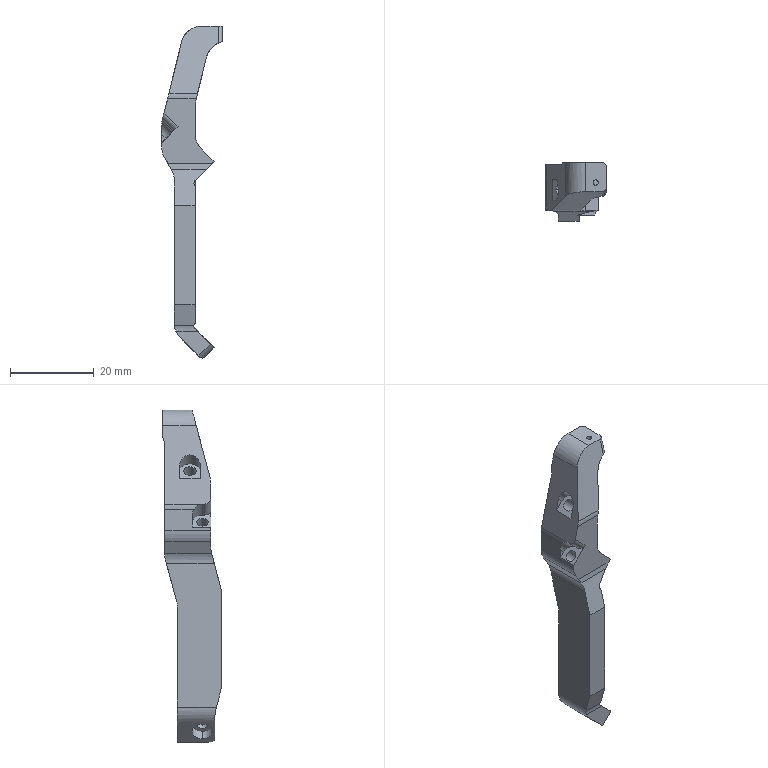NC program | NX | posted by the shop | part box 14.5 x 14 x 79.438 mm
Lines 12095 to 13169 of 13169:
T04 M6 ( D4-12-D4-50-3T-rough )
M41
M51
G90 G54 G00 B90. C225.
M40
M50
G54 G00 X-166.572 Y-9.003 S3000 M03
G43 H04 Z-115.926 M08
Z-148.07
G01 Z-150.07 F400.
Y-13.003
Y-15.568
G03 X-166.122 Y-16.018 R0.45
X-165.672 Y-15.568 R0.45
G01 Y-13.003
Y-9.003
Z-148.07
G00 X-166.572 Z-148.17
G01 Z-150.17
Y-13.003
Y-15.568
G03 X-166.122 Y-16.018 R0.45
X-165.672 Y-15.568 R0.45
G01 Y-13.003
Y-9.003
Z-148.17
G00 X-166.572 Z-148.27
G01 Z-150.27
Y-13.003
Y-15.568
G03 X-166.122 Y-16.018 R0.45
X-165.672 Y-15.568 R0.45
G01 Y-13.003
Y-9.003
Z-148.27
G00 X-166.572 Z-148.37
G01 Z-150.37
Y-13.003
Y-15.568
G03 X-166.122 Y-16.018 R0.45
X-165.672 Y-15.568 R0.45
G01 Y-13.003
Y-9.003
Z-148.37
G00 X-166.572 Z-148.47
G01 Z-150.47
Y-13.003
Y-15.568
G03 X-166.122 Y-16.018 R0.45
X-165.672 Y-15.568 R0.45
G01 Y-13.003
Y-9.003
Z-148.47
G00 X-166.572 Z-148.57
G01 Z-150.57
Y-13.003
Y-15.568
G03 X-166.122 Y-16.018 R0.45
X-165.672 Y-15.568 R0.45
G01 Y-13.003
Y-9.003
Z-148.57
G00 X-166.572 Z-148.67
G01 Z-150.67
Y-13.003
Y-15.568
G03 X-166.122 Y-16.018 R0.45
X-165.672 Y-15.568 R0.45
G01 Y-13.003
Y-9.003
Z-148.67
G00 X-166.572 Z-148.77
G01 Z-150.77
Y-13.003
Y-15.568
G03 X-166.122 Y-16.018 R0.45
X-165.672 Y-15.568 R0.45
G01 Y-13.003
Y-9.003
Z-148.77
G00 X-166.572 Z-148.87
G01 Z-150.87
Y-13.003
Y-15.568
G03 X-166.122 Y-16.018 R0.45
X-165.672 Y-15.568 R0.45
G01 Y-13.003
Y-9.003
Z-148.87
G00 X-166.572 Z-148.97
G01 Z-150.97
Y-13.003
Y-15.568
G03 X-166.122 Y-16.018 R0.45
X-165.672 Y-15.568 R0.45
G01 Y-13.003
Y-9.003
Z-148.97
G00 X-166.572 Z-149.07
G01 Z-151.07
Y-13.003
Y-15.568
G03 X-166.122 Y-16.018 R0.45
X-165.672 Y-15.568 R0.45
G01 Y-13.003
Y-9.003
Z-149.07
G00 X-166.572 Z-149.17
G01 Z-151.17
Y-13.003
Y-15.568
G03 X-166.122 Y-16.018 R0.45
X-165.672 Y-15.568 R0.45
G01 Y-13.003
Y-9.003
Z-149.17
G00 X-166.572 Z-149.27
G01 Z-151.27
Y-13.003
Y-15.568
G03 X-166.122 Y-16.018 R0.45
X-165.672 Y-15.568 R0.45
G01 Y-13.003
Y-9.003
Z-149.27
G00 X-166.572 Z-149.37
G01 Z-151.37
Y-13.003
Y-15.568
G03 X-166.122 Y-16.018 R0.45
X-165.672 Y-15.568 R0.45
G01 Y-13.003
Y-9.003
Z-149.37
G00 X-166.572 Z-149.47
G01 Z-151.47
Y-13.003
Y-15.568
G03 X-166.122 Y-16.018 R0.45
X-165.672 Y-15.568 R0.45
G01 Y-13.003
Y-9.003
Z-149.47
G00 X-166.572 Z-149.57
G01 Z-151.57
Y-13.003
Y-15.568
G03 X-166.122 Y-16.018 R0.45
X-165.672 Y-15.568 R0.45
G01 Y-13.003
Y-9.003
Z-149.57
G00 X-166.572 Z-149.67
G01 Z-151.67
Y-13.003
Y-15.568
G03 X-166.122 Y-16.018 R0.45
X-165.672 Y-15.568 R0.45
G01 Y-13.003
Y-9.003
Z-149.67
G00 X-166.572 Z-149.77
G01 Z-151.77
Y-13.003
Y-15.568
G03 X-166.122 Y-16.018 R0.45
X-165.672 Y-15.568 R0.45
G01 Y-13.003
Y-9.003
Z-149.77
G00 X-166.572 Z-149.87
G01 Z-151.87
Y-13.003
Y-15.568
G03 X-166.122 Y-16.018 R0.45
X-165.672 Y-15.568 R0.45
G01 Y-13.003
Y-9.003
Z-149.87
G00 X-166.572 Z-149.97
G01 Z-151.97
Y-13.003
Y-15.568
G03 X-166.122 Y-16.018 R0.45
X-165.672 Y-15.568 R0.45
G01 Y-13.003
Y-9.003
Z-149.97
G00 X-166.572 Z-150.07
G01 Z-152.07
Y-13.003
Y-15.568
G03 X-166.122 Y-16.018 R0.45
X-165.672 Y-15.568 R0.45
G01 Y-13.003
Y-9.003
Z-150.07
G00 X-166.572 Z-150.17
G01 Z-152.17
Y-13.003
Y-15.568
G03 X-166.122 Y-16.018 R0.45
X-165.672 Y-15.568 R0.45
G01 Y-13.003
Y-9.003
Z-150.17
G00 X-166.572 Z-150.27
G01 Z-152.27
Y-13.003
Y-15.568
G03 X-166.122 Y-16.018 R0.45
X-165.672 Y-15.568 R0.45
G01 Y-13.003
Y-9.003
Z-150.27
G00 X-166.572 Z-150.37
G01 Z-152.37
Y-13.003
Y-15.568
G03 X-166.122 Y-16.018 R0.45
X-165.672 Y-15.568 R0.45
G01 Y-13.003
Y-9.003
Z-150.37
G00 X-166.572 Z-150.47
G01 Z-152.47
Y-13.003
Y-15.568
G03 X-166.122 Y-16.018 R0.45
X-165.672 Y-15.568 R0.45
G01 Y-13.003
Y-9.003
Z-150.47
G00 X-166.572 Z-150.57
G01 Z-152.57
Y-13.003
Y-15.568
G03 X-166.122 Y-16.018 R0.45
X-165.672 Y-15.568 R0.45
G01 Y-13.003
Y-9.003
Z-150.57
G00 X-166.572 Z-150.67
G01 Z-152.67
Y-13.003
Y-15.568
G03 X-166.122 Y-16.018 R0.45
X-165.672 Y-15.568 R0.45
G01 Y-13.003
Y-9.003
Z-150.67
G00 X-166.572 Z-150.77
G01 Z-152.77
Y-13.003
Y-15.568
G03 X-166.122 Y-16.018 R0.45
X-165.672 Y-15.568 R0.45
G01 Y-13.003
Y-9.003
Z-150.77
G00 X-166.572 Z-150.87
G01 Z-152.87
Y-13.003
Y-15.568
G03 X-166.122 Y-16.018 R0.45
X-165.672 Y-15.568 R0.45
G01 Y-13.003
Y-9.003
Z-150.87
G00 X-166.572 Z-150.97
G01 Z-152.97
Y-13.003
Y-15.568
G03 X-166.122 Y-16.018 R0.45
X-165.672 Y-15.568 R0.45
G01 Y-13.003
Y-9.003
Z-150.97
G00 X-166.572 Z-151.07
G01 Z-153.07
Y-13.003
Y-15.568
G03 X-166.122 Y-16.018 R0.45
X-165.672 Y-15.568 R0.45
G01 Y-13.003
Y-9.003
Z-151.07
G00 X-166.572 Z-151.17
G01 Z-153.17
Y-13.003
Y-15.568
G03 X-166.122 Y-16.018 R0.45
X-165.672 Y-15.568 R0.45
G01 Y-13.003
Y-9.003
Z-151.17
G00 X-166.572 Z-151.27
G01 Z-153.27
Y-13.003
Y-15.568
G03 X-166.122 Y-16.018 R0.45
X-165.672 Y-15.568 R0.45
G01 Y-13.003
Y-9.003
Z-151.27
G00 X-166.572 Z-151.37
G01 Z-153.37
Y-13.003
Y-15.568
G03 X-166.122 Y-16.018 R0.45
X-165.672 Y-15.568 R0.45
G01 Y-13.003
Y-9.003
Z-151.37
G00 X-166.572 Z-151.42
G01 Z-153.42
Y-13.003
Y-15.568
G03 X-166.122 Y-16.018 R0.45
X-165.672 Y-15.568 R0.45
G01 Y-13.003
Y-9.003
Z-151.42
G00 Z-115.926
G00 X-175.172 Y-11.221
Z-153.57
G01 Z-155.57 F400.
G03 X-173.172 Y-9.221 R2.
G02 X-169.622 Y-5.671 R3.55
G01 X-169.122
G03 X-168.672 Y-5.221 R0.45
G01 Y-5.211
Y-2.711
G03 X-170.672 Y-0.711 R2.
G01 Z-153.57
G00 X-175.172 Y-11.221 Z-153.67
G01 Z-155.67
G03 X-173.172 Y-9.221 R2.
G02 X-169.622 Y-5.671 R3.55
G01 X-169.122
G03 X-168.672 Y-5.221 R0.45
G01 Y-5.211
Y-2.711
G03 X-170.672 Y-0.711 R2.
G01 Z-153.67
G00 X-175.172 Y-11.221 Z-153.77
G01 Z-155.77
G03 X-173.172 Y-9.221 R2.
G02 X-169.622 Y-5.671 R3.55
G01 X-169.122
G03 X-168.672 Y-5.221 R0.45
G01 Y-5.211
Y-2.711
G03 X-170.672 Y-0.711 R2.
G01 Z-153.77
G00 X-175.172 Y-11.221 Z-153.87
G01 Z-155.87
G03 X-173.172 Y-9.221 R2.
G02 X-169.622 Y-5.671 R3.55
G01 X-169.122
G03 X-168.672 Y-5.221 R0.45
G01 Y-5.211
Y-2.711
G03 X-170.672 Y-0.711 R2.
G01 Z-153.87
G00 X-175.172 Y-11.221 Z-153.97
G01 Z-155.97
G03 X-173.172 Y-9.221 R2.
G02 X-169.622 Y-5.671 R3.55
G01 X-169.122
G03 X-168.672 Y-5.221 R0.45
G01 Y-5.211
Y-2.711
G03 X-170.672 Y-0.711 R2.
G01 Z-153.97
G00 X-175.172 Y-11.221 Z-154.07
G01 Z-156.07
G03 X-173.172 Y-9.221 R2.
G02 X-169.622 Y-5.671 R3.55
G01 X-169.122
G03 X-168.672 Y-5.221 R0.45
G01 Y-5.211
Y-2.711
G03 X-170.672 Y-0.711 R2.
G01 Z-154.07
G00 X-175.172 Y-11.221 Z-154.17
G01 Z-156.17
G03 X-173.172 Y-9.221 R2.
G02 X-169.622 Y-5.671 R3.55
G01 X-169.122
G03 X-168.672 Y-5.221 R0.45
G01 Y-5.211
Y-2.711
G03 X-170.672 Y-0.711 R2.
G01 Z-154.17
G00 X-175.172 Y-11.221 Z-154.27
G01 Z-156.27
G03 X-173.172 Y-9.221 R2.
G02 X-169.622 Y-5.671 R3.55
G01 X-169.122
G03 X-168.672 Y-5.221 R0.45
G01 Y-5.211
Y-2.711
G03 X-170.672 Y-0.711 R2.
G01 Z-154.27
G00 X-175.172 Y-11.221 Z-154.37
G01 Z-156.37
G03 X-173.172 Y-9.221 R2.
G02 X-169.622 Y-5.671 R3.55
G01 X-169.122
G03 X-168.672 Y-5.221 R0.45
G01 Y-5.211
Y-2.711
G03 X-170.672 Y-0.711 R2.
G01 Z-154.37
G00 X-175.172 Y-11.221 Z-154.47
G01 Z-156.47
G03 X-173.172 Y-9.221 R2.
G02 X-169.622 Y-5.671 R3.55
G01 X-169.122
G03 X-168.672 Y-5.221 R0.45
G01 Y-5.211
Y-2.711
G03 X-170.672 Y-0.711 R2.
G01 Z-154.47
G00 X-175.172 Y-11.221 Z-154.57
G01 Z-156.57
G03 X-173.172 Y-9.221 R2.
G02 X-169.622 Y-5.671 R3.55
G01 X-169.122
G03 X-168.672 Y-5.221 R0.45
G01 Y-5.211
Y-2.711
G03 X-170.672 Y-0.711 R2.
G01 Z-154.57
G00 X-175.172 Y-11.221 Z-154.67
G01 Z-156.67
G03 X-173.172 Y-9.221 R2.
G02 X-169.622 Y-5.671 R3.55
G01 X-169.122
G03 X-168.672 Y-5.221 R0.45
G01 Y-5.211
Y-2.711
G03 X-170.672 Y-0.711 R2.
G01 Z-154.67
G00 X-175.172 Y-11.221 Z-154.77
G01 Z-156.77
G03 X-173.172 Y-9.221 R2.
G02 X-169.622 Y-5.671 R3.55
G01 X-169.122
G03 X-168.672 Y-5.221 R0.45
G01 Y-5.211
Y-2.711
G03 X-170.672 Y-0.711 R2.
G01 Z-154.77
G00 X-175.172 Y-11.221 Z-154.87
G01 Z-156.87
G03 X-173.172 Y-9.221 R2.
G02 X-169.622 Y-5.671 R3.55
G01 X-169.122
G03 X-168.672 Y-5.221 R0.45
G01 Y-5.211
Y-2.711
G03 X-170.672 Y-0.711 R2.
G01 Z-154.87
G00 X-175.172 Y-11.221 Z-154.97
G01 Z-156.97
G03 X-173.172 Y-9.221 R2.
G02 X-169.622 Y-5.671 R3.55
G01 X-169.122
G03 X-168.672 Y-5.221 R0.45
G01 Y-5.211
Y-2.711
G03 X-170.672 Y-0.711 R2.
G01 Z-154.97
G00 X-175.172 Y-11.221 Z-155.07
G01 Z-157.07
G03 X-173.172 Y-9.221 R2.
G02 X-169.622 Y-5.671 R3.55
G01 X-169.122
G03 X-168.672 Y-5.221 R0.45
G01 Y-5.211
Y-2.711
G03 X-170.672 Y-0.711 R2.
G01 Z-155.07
G00 X-175.172 Y-11.221 Z-155.17
G01 Z-157.17
G03 X-173.172 Y-9.221 R2.
G02 X-169.622 Y-5.671 R3.55
G01 X-169.122
G03 X-168.672 Y-5.221 R0.45
G01 Y-5.211
Y-2.711
G03 X-170.672 Y-0.711 R2.
G01 Z-155.17
G00 X-175.172 Y-11.221 Z-155.27
G01 Z-157.27
G03 X-173.172 Y-9.221 R2.
G02 X-169.622 Y-5.671 R3.55
G01 X-169.122
G03 X-168.672 Y-5.221 R0.45
G01 Y-5.211
Y-2.711
G03 X-170.672 Y-0.711 R2.
G01 Z-155.27
G00 X-175.172 Y-11.221 Z-155.37
G01 Z-157.37
G03 X-173.172 Y-9.221 R2.
G02 X-169.622 Y-5.671 R3.55
G01 X-169.122
G03 X-168.672 Y-5.221 R0.45
G01 Y-5.211
Y-2.711
G03 X-170.672 Y-0.711 R2.
G01 Z-155.37
G00 X-175.172 Y-11.221 Z-155.47
G01 Z-157.47
G03 X-173.172 Y-9.221 R2.
G02 X-169.622 Y-5.671 R3.55
G01 X-169.122
G03 X-168.672 Y-5.221 R0.45
G01 Y-5.211
Y-2.711
G03 X-170.672 Y-0.711 R2.
G01 Z-155.47
G00 X-175.172 Y-11.221 Z-155.57
G01 Z-157.57
G03 X-173.172 Y-9.221 R2.
G02 X-169.622 Y-5.671 R3.55
G01 X-169.122
G03 X-168.672 Y-5.221 R0.45
G01 Y-5.211
Y-2.711
G03 X-170.672 Y-0.711 R2.
G01 Z-155.57
G00 X-175.172 Y-11.221 Z-155.67
G01 Z-157.67
G03 X-173.172 Y-9.221 R2.
G02 X-169.622 Y-5.671 R3.55
G01 X-169.122
G03 X-168.672 Y-5.221 R0.45
G01 Y-5.211
Y-2.711
G03 X-170.672 Y-0.711 R2.
G01 Z-155.67
G00 X-175.172 Y-11.221 Z-155.77
G01 Z-157.77
G03 X-173.172 Y-9.221 R2.
G02 X-169.622 Y-5.671 R3.55
G01 X-169.122
G03 X-168.672 Y-5.221 R0.45
G01 Y-5.211
Y-2.711
G03 X-170.672 Y-0.711 R2.
G01 Z-155.77
G00 X-175.172 Y-11.221 Z-155.87
G01 Z-157.87
G03 X-173.172 Y-9.221 R2.
G02 X-169.622 Y-5.671 R3.55
G01 X-169.122
G03 X-168.672 Y-5.221 R0.45
G01 Y-5.211
Y-2.711
G03 X-170.672 Y-0.711 R2.
G01 Z-155.87
G00 X-175.172 Y-11.221 Z-155.97
G01 Z-157.97
G03 X-173.172 Y-9.221 R2.
G02 X-169.622 Y-5.671 R3.55
G01 X-169.122
G03 X-168.672 Y-5.221 R0.45
G01 Y-5.211
Y-2.711
G03 X-170.672 Y-0.711 R2.
G01 Z-155.97
G00 X-175.172 Y-11.221 Z-156.07
G01 Z-158.07
G03 X-173.172 Y-9.221 R2.
G02 X-169.622 Y-5.671 R3.55
G01 X-169.122
G03 X-168.672 Y-5.221 R0.45
G01 Y-5.211
Y-2.711
G03 X-170.672 Y-0.711 R2.
G01 Z-156.07
G00 X-175.172 Y-11.221 Z-156.17
G01 Z-158.17
G03 X-173.172 Y-9.221 R2.
G02 X-169.622 Y-5.671 R3.55
G01 X-169.122
G03 X-168.672 Y-5.221 R0.45
G01 Y-5.211
Y-2.711
G03 X-170.672 Y-0.711 R2.
G01 Z-156.17
G00 X-175.172 Y-11.221 Z-156.27
G01 Z-158.27
G03 X-173.172 Y-9.221 R2.
G02 X-169.622 Y-5.671 R3.55
G01 X-169.122
G03 X-168.672 Y-5.221 R0.45
G01 Y-5.211
Y-2.711
G03 X-170.672 Y-0.711 R2.
G01 Z-156.27
G00 X-175.172 Y-11.221 Z-156.37
G01 Z-158.37
G03 X-173.172 Y-9.221 R2.
G02 X-169.622 Y-5.671 R3.55
G01 X-169.122
G03 X-168.672 Y-5.221 R0.45
G01 Y-5.211
Y-2.711
G03 X-170.672 Y-0.711 R2.
G01 Z-156.37
G00 X-175.172 Y-11.221 Z-156.47
G01 Z-158.47
G03 X-173.172 Y-9.221 R2.
G02 X-169.622 Y-5.671 R3.55
G01 X-169.122
G03 X-168.672 Y-5.221 R0.45
G01 Y-5.211
Y-2.711
G03 X-170.672 Y-0.711 R2.
G01 Z-156.47
G00 X-175.172 Y-11.221 Z-156.57
G01 Z-158.57
G03 X-173.172 Y-9.221 R2.
G02 X-169.622 Y-5.671 R3.55
G01 X-169.122
G03 X-168.672 Y-5.221 R0.45
G01 Y-5.211
Y-2.711
G03 X-170.672 Y-0.711 R2.
G01 Z-156.57
G00 X-175.172 Y-11.221 Z-156.67
G01 Z-158.67
G03 X-173.172 Y-9.221 R2.
G02 X-169.622 Y-5.671 R3.55
G01 X-169.122
G03 X-168.672 Y-5.221 R0.45
G01 Y-5.211
Y-2.711
G03 X-170.672 Y-0.711 R2.
G01 Z-156.67
G00 X-175.172 Y-11.221 Z-156.77
G01 Z-158.77
G03 X-173.172 Y-9.221 R2.
G02 X-169.622 Y-5.671 R3.55
G01 X-169.122
G03 X-168.672 Y-5.221 R0.45
G01 Y-5.211
Y-2.711
G03 X-170.672 Y-0.711 R2.
G01 Z-156.77
G00 X-175.172 Y-11.221 Z-156.87
G01 Z-158.87
G03 X-173.172 Y-9.221 R2.
G02 X-169.622 Y-5.671 R3.55
G01 X-169.122
G03 X-168.672 Y-5.221 R0.45
G01 Y-5.211
Y-2.711
G03 X-170.672 Y-0.711 R2.
G01 Z-156.87
G00 X-175.172 Y-11.221 Z-156.97
G01 Z-158.97
G03 X-173.172 Y-9.221 R2.
G02 X-169.622 Y-5.671 R3.55
G01 X-169.122
G03 X-168.672 Y-5.221 R0.45
G01 Y-5.211
Y-2.711
G03 X-170.672 Y-0.711 R2.
G01 Z-156.97
G00 X-175.172 Y-11.221 Z-157.07
G01 Z-159.07
G03 X-173.172 Y-9.221 R2.
G02 X-169.622 Y-5.671 R3.55
G01 X-169.122
G03 X-168.672 Y-5.221 R0.45
G01 Y-5.211
Y-2.711
G03 X-170.672 Y-0.711 R2.
G01 Z-157.07
G00 X-175.172 Y-11.221 Z-157.17
G01 Z-159.17
G03 X-173.172 Y-9.221 R2.
G02 X-169.622 Y-5.671 R3.55
G01 X-169.122
G03 X-168.672 Y-5.221 R0.45
G01 Y-5.211
Y-2.711
G03 X-170.672 Y-0.711 R2.
G01 Z-157.17
G00 X-175.172 Y-11.221 Z-157.27
G01 Z-159.27
G03 X-173.172 Y-9.221 R2.
G02 X-169.622 Y-5.671 R3.55
G01 X-169.122
G03 X-168.672 Y-5.221 R0.45
G01 Y-5.211
Y-2.711
G03 X-170.672 Y-0.711 R2.
G01 Z-157.27
G00 X-175.172 Y-11.221 Z-157.37
G01 Z-159.37
G03 X-173.172 Y-9.221 R2.
G02 X-169.622 Y-5.671 R3.55
G01 X-169.122
G03 X-168.672 Y-5.221 R0.45
G01 Y-5.211
Y-2.711
G03 X-170.672 Y-0.711 R2.
G01 Z-157.37
G00 X-175.172 Y-11.221 Z-157.47
G01 Z-159.47
G03 X-173.172 Y-9.221 R2.
G02 X-169.622 Y-5.671 R3.55
G01 X-169.122
G03 X-168.672 Y-5.221 R0.45
G01 Y-5.211
Y-2.711
G03 X-170.672 Y-0.711 R2.
G01 Z-157.47
G00 X-175.172 Y-11.221 Z-157.57
G01 Z-159.57
G03 X-173.172 Y-9.221 R2.
G02 X-169.622 Y-5.671 R3.55
G01 X-169.122
G03 X-168.672 Y-5.221 R0.45
G01 Y-5.211
Y-2.711
G03 X-170.672 Y-0.711 R2.
G01 Z-157.57
G00 X-175.172 Y-11.221 Z-157.67
G01 Z-159.67
G03 X-173.172 Y-9.221 R2.
G02 X-169.622 Y-5.671 R3.55
G01 X-169.122
G03 X-168.672 Y-5.221 R0.45
G01 Y-5.211
Y-2.711
G03 X-170.672 Y-0.711 R2.
G01 Z-157.67
G00 X-175.172 Y-11.221 Z-157.77
G01 Z-159.77
G03 X-173.172 Y-9.221 R2.
G02 X-169.622 Y-5.671 R3.55
G01 X-169.122
G03 X-168.672 Y-5.221 R0.45
G01 Y-5.211
Y-2.711
G03 X-170.672 Y-0.711 R2.
G01 Z-157.77
G00 X-175.172 Y-11.221 Z-157.87
G01 Z-159.87
G03 X-173.172 Y-9.221 R2.
G02 X-169.622 Y-5.671 R3.55
G01 X-169.122
G03 X-168.672 Y-5.221 R0.45
G01 Y-5.211
Y-2.711
G03 X-170.672 Y-0.711 R2.
G01 Z-157.87
G00 X-175.172 Y-11.221 Z-157.97
G01 Z-159.97
G03 X-173.172 Y-9.221 R2.
G02 X-169.622 Y-5.671 R3.55
G01 X-169.122
G03 X-168.672 Y-5.221 R0.45
G01 Y-5.211
Y-2.711
G03 X-170.672 Y-0.711 R2.
G01 Z-157.97
G00 X-175.172 Y-11.221 Z-158.07
G01 Z-160.07
G03 X-173.172 Y-9.221 R2.
G02 X-169.622 Y-5.671 R3.55
G01 X-169.122
G03 X-168.672 Y-5.221 R0.45
G01 Y-5.211
Y-2.711
G03 X-170.672 Y-0.711 R2.
G01 Z-158.07
G00 X-175.172 Y-11.221 Z-158.17
G01 Z-160.17
G03 X-173.172 Y-9.221 R2.
G02 X-169.622 Y-5.671 R3.55
G01 X-169.122
G03 X-168.672 Y-5.221 R0.45
G01 Y-5.211
Y-2.711
G03 X-170.672 Y-0.711 R2.
G01 Z-158.17
G00 X-175.172 Y-11.221 Z-158.27
G01 Z-160.27
G03 X-173.172 Y-9.221 R2.
G02 X-169.622 Y-5.671 R3.55
G01 X-169.122
G03 X-168.672 Y-5.221 R0.45
G01 Y-5.211
Y-2.711
G03 X-170.672 Y-0.711 R2.
G01 Z-158.27
G00 X-175.172 Y-11.221 Z-158.37
G01 Z-160.37
G03 X-173.172 Y-9.221 R2.
G02 X-169.622 Y-5.671 R3.55
G01 X-169.122
G03 X-168.672 Y-5.221 R0.45
G01 Y-5.211
Y-2.711
G03 X-170.672 Y-0.711 R2.
G01 Z-158.37
G00 X-175.172 Y-11.221 Z-158.42
G01 Z-160.42
G03 X-173.172 Y-9.221 R2.
G02 X-169.622 Y-5.671 R3.55
G01 X-169.122
G03 X-168.672 Y-5.221 R0.45
G01 Y-5.211
Y-2.711
G03 X-170.672 Y-0.711 R2.
G01 Z-158.42
G00 Z-115.926
M09
M05
G91 G28 Z0.
G91 G28 X0. Y0.
M01
N04
G17 G40 G80 G94
T05 M6 ( D4-12-D4-50-3T-finish )
M41
M51
G90 G54 G00 B90. C225.
M40
M50
G54 G00 X-166.622 Y-9.003 S3000 M03
G43 H05 Z-115.976 M08
Z-151.47
G01 Z-153.47 F600.
Y-13.003
Y-15.568
G03 X-166.122 Y-16.068 R0.5
X-165.622 Y-15.568 R0.5
G01 Y-13.003
Y-9.003
Z-151.47
G00 Z-115.976
X-166.622
Z-151.47
G01 Z-153.47
Y-13.003
Y-15.568
G03 X-166.122 Y-16.068 R0.5
X-165.622 Y-15.568 R0.5
G01 Y-13.003
Y-9.003
Z-151.47
G00 Z-115.976
G00 X-175.122 Y-11.221
Z-158.47
G01 Z-160.47 F600.
G03 X-173.122 Y-9.221 R2.
G02 X-169.622 Y-5.721 R3.5
G01 X-169.122
G03 X-168.622 Y-5.221 R0.5
G01 Y-5.211
Y-2.711
G03 X-170.622 Y-0.711 R2.
G01 Z-158.47
G00 Z-115.976
X-175.122 Y-11.221
Z-158.47
G01 Z-160.47
G03 X-173.122 Y-9.221 R2.
G02 X-169.622 Y-5.721 R3.5
G01 X-169.122
G03 X-168.622 Y-5.221 R0.5
G01 Y-5.211
Y-2.711
G03 X-170.622 Y-0.711 R2.
G01 Z-158.47
G00 Z-115.976
G91 G28 Z0.
M01
M41
M51
G90 G54 G00 B90. C90.
M40
M50
G54 G00 X-178.672 Y-16.709 S3000 M03
G43 H05 Z-135.64 M08
Z-168.99
G01 Z-171.99 F600.
X-173.672
G03 X-172.672 Y-15.709 R1.
G01 Y-4.088
X-171.667 Y-0.337
X-165.172
Y-0.023
X-164.072
Y15.216
X-170.172
Y17.936
X-161.072
Y4.343
G02 X-161.21 Y3.295 R4.05
G01 X-163.869 Y-6.63
G03 X-164.072 Y-8.17 R5.95
G01 Y-31.089
X-171.734
X-172.672 Y-27.588
Y-15.709
X-169.672
Y-4.483
X-169.365 Y-3.337
X-166.093
X-166.767 Y-5.853
G03 X-167.072 Y-8.17 R8.95
G01 Y-28.089
X-169.432
X-169.672 Y-27.193
Y-15.709
Y-14.709
G03 X-170.672 Y-13.709 R1.
G01 X-178.672
Z-168.99
G00 Z-135.64
Y-16.709
Z-169.19
G01 Z-172.19
X-173.672
G03 X-172.672 Y-15.709 R1.
G01 Y-4.088
X-171.667 Y-0.337
X-165.172
Y-0.023
X-164.072
Y15.216
X-170.172
Y17.936
X-161.072
Y4.343
G02 X-161.21 Y3.295 R4.05
G01 X-163.869 Y-6.63
G03 X-164.072 Y-8.17 R5.95
G01 Y-31.089
X-171.734
X-172.672 Y-27.588
Y-15.709
X-169.672
Y-4.483
X-169.365 Y-3.337
X-166.093
X-166.767 Y-5.853
G03 X-167.072 Y-8.17 R8.95
G01 Y-28.089
X-169.432
X-169.672 Y-27.193
Y-15.709
Y-14.709
G03 X-170.672 Y-13.709 R1.
G01 X-178.672
Z-169.19
G00 Z-135.64
G00 Y-16.709
Z-169.19
G01 Z-172.24 F600.
X-173.672
G03 X-172.672 Y-15.709 R1.
G01 Y-4.088
X-171.667 Y-0.337
X-165.172
Y-0.023
X-164.072
Y15.216
X-170.172
Y17.936
X-161.072
Y4.343
G02 X-161.21 Y3.295 R4.05
G01 X-163.869 Y-6.63
G03 X-164.072 Y-8.17 R5.95
G01 Y-31.089
X-171.734
X-172.672 Y-27.588
Y-15.709
X-169.672
Y-4.483
X-169.365 Y-3.337
X-166.093
X-166.767 Y-5.853
G03 X-167.072 Y-8.17 R8.95
G01 Y-28.089
X-169.432
X-169.672 Y-27.193
Y-15.709
Y-14.709
G03 X-170.672 Y-13.709 R1.
G01 X-178.672
Z-169.19
G00 Z-135.64
G00 X-175.122 Y15.166 Z-142.19
Z-169.24
G01 Z-172.24 F600.
X-171.122
X-166.122
G02 X-164.122 Y13.166 R2.
G01 Y0.613
G02 X-166.122 Y-1.387 R2.
G01 X-172.396
X-176.396
Z-169.24
G00 Z-142.19
M09
M05
G91 G28 Z0.
G91 G28 X0. Y0.
M01
N05
G17 G40 G80 G94
T06 M6 ( Chamfer D4-90deg )
M41
M51
G90 G54 G00 B90. C180.
M40
M50
G54 G00 X-164.422 Y-5.616 S2500 M03
G43 H06 Z-99.903 M08
G98 G81 Z-134.703 R-130.903 F80.
G80
G91 G28 Z0.
M01
M41
M51
G90 G54 G00 B90. C225.
M40
M50
G54 G00 X-166.122 Y-15.568 S2500 M03
G43 H06 Z-107.249 M08
G81 Z-154.47 R-149.47 F80.
G80
G00 X-169.122 Y-5.221 Z-107.249
G81 Z-161.47 R-157.47 F80.
G80
G91 G28 Z0.
M01
M41
M51
G90 G54 G00 B90. C315.
M40
M50
G54 G00 X-169.122 Y25.964 S2500 M03
G43 H06 Z-106.897 M08
G81 Z-147.861 R-143.861 F80.
G80
M09
M05
G91 G28 Z0.
G91 G28 X0. Y0.
M41
M51
G00 G90 B0.0 C0.0
M40
M50
M01
M30